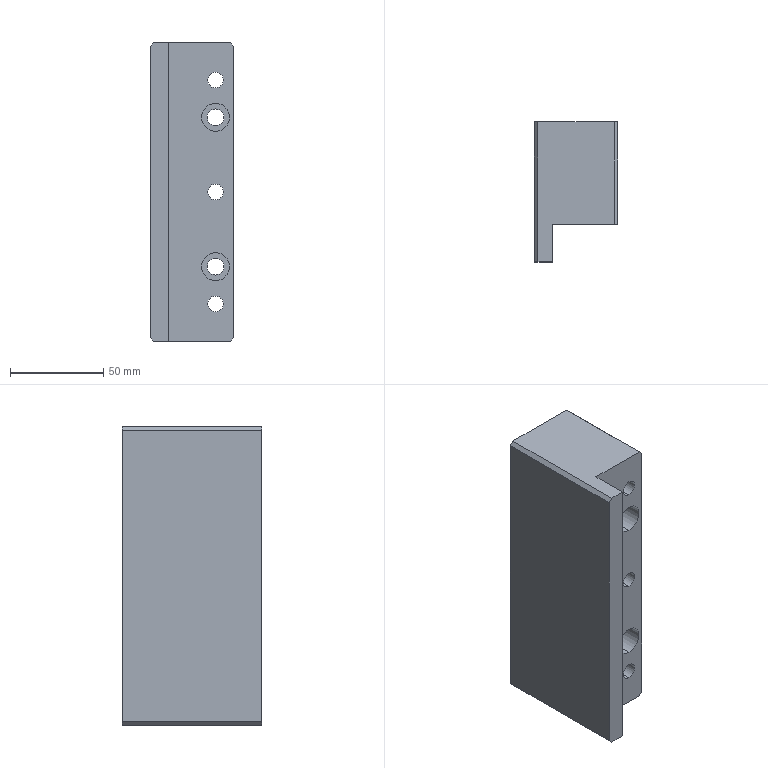Part | SolidWorks | features HoleWzd 2, Chamfer 1, Cut 1, Extrusion 1 | 1 solid | 28 faces | box 44.75 x 75 x 160 mm | volume 399871 mm3 | cylinder 14 | plane 14 | commonest cylinder face diameters 8.5 x6 9 x4 15 x4
STEP:
#1=CARTESIAN_POINT('',(12.625,60.,47.5));
#2=VERTEX_POINT('',#1);
#3=CARTESIAN_POINT('',(12.625,60.,32.5));
#4=VERTEX_POINT('',#3);
#5=CARTESIAN_POINT('',(12.625,60.,40.));
#6=DIRECTION('',(0.,-1.,0.));
#7=DIRECTION('',(0.,0.,-1.));
#8=AXIS2_PLACEMENT_3D('',#5,#6,#7);
#9=CIRCLE('',#8,7.5);
#10=EDGE_CURVE('',#2,#4,#9,.T.);
#11=ORIENTED_EDGE('',*,*,#10,.F.);
#12=CARTESIAN_POINT('',(12.625,20.,47.5));
#13=VERTEX_POINT('',#12);
#14=CARTESIAN_POINT('',(12.625,20.,47.5));
#15=DIRECTION('',(0.,-1.,0.));
#16=VECTOR('',#15,1000.);
#17=LINE('',#14,#16);
#18=EDGE_CURVE('',#2,#13,#17,.T.);
#19=ORIENTED_EDGE('',*,*,#18,.T.);
#20=CARTESIAN_POINT('',(12.625,20.,32.5));
#21=VERTEX_POINT('',#20);
#22=CARTESIAN_POINT('',(12.625,20.,40.));
#23=DIRECTION('',(0.,-1.,0.));
#24=DIRECTION('',(0.,0.,-1.));
#25=AXIS2_PLACEMENT_3D('',#22,#23,#24);
#26=CIRCLE('',#25,7.5);
#27=EDGE_CURVE('',#13,#21,#26,.T.);
#28=ORIENTED_EDGE('',*,*,#27,.T.);
#29=CARTESIAN_POINT('',(12.625,20.,32.5));
#30=DIRECTION('',(0.,-1.,0.));
#31=VECTOR('',#30,1000.);
#32=LINE('',#29,#31);
#33=EDGE_CURVE('',#4,#21,#32,.T.);
#34=ORIENTED_EDGE('',*,*,#33,.F.);
#35=EDGE_LOOP('',(#11,#19,#28,#34));
#36=FACE_OUTER_BOUND('',#35,.T.);
#37=CARTESIAN_POINT('',(12.625,20.,40.));
#38=DIRECTION('',(0.,-1.,0.));
#39=DIRECTION('',(0.,0.,-1.));
#40=AXIS2_PLACEMENT_3D('',#37,#38,#39);
#41=CYLINDRICAL_SURFACE('',#40,7.5);
#42=ADVANCED_FACE('',(#36),#41,.F.);
#43=CARTESIAN_POINT('',(12.625,75.,44.5));
#44=VERTEX_POINT('',#43);
#45=CARTESIAN_POINT('',(12.625,75.,35.5));
#46=VERTEX_POINT('',#45);
#47=CARTESIAN_POINT('',(12.625,75.,40.));
#48=DIRECTION('',(0.,-1.,0.));
#49=DIRECTION('',(0.,0.,-1.));
#50=AXIS2_PLACEMENT_3D('',#47,#48,#49);
#51=CIRCLE('',#50,4.5);
#52=EDGE_CURVE('',#44,#46,#51,.T.);
#53=ORIENTED_EDGE('',*,*,#52,.F.);
#54=CARTESIAN_POINT('',(12.625,60.,44.5));
#55=VERTEX_POINT('',#54);
#56=CARTESIAN_POINT('',(12.625,20.,44.5));
#57=DIRECTION('',(0.,-1.,0.));
#58=VECTOR('',#57,1000.);
#59=LINE('',#56,#58);
#60=EDGE_CURVE('',#44,#55,#59,.T.);
#61=ORIENTED_EDGE('',*,*,#60,.T.);
#62=CARTESIAN_POINT('',(12.625,60.,35.5));
#63=VERTEX_POINT('',#62);
#64=CARTESIAN_POINT('',(12.625,60.,40.));
#65=DIRECTION('',(0.,-1.,0.));
#66=DIRECTION('',(0.,0.,-1.));
#67=AXIS2_PLACEMENT_3D('',#64,#65,#66);
#68=CIRCLE('',#67,4.5);
#69=EDGE_CURVE('',#55,#63,#68,.T.);
#70=ORIENTED_EDGE('',*,*,#69,.T.);
#71=CARTESIAN_POINT('',(12.625,20.,35.5));
#72=DIRECTION('',(0.,-1.,0.));
#73=VECTOR('',#72,1000.);
#74=LINE('',#71,#73);
#75=EDGE_CURVE('',#46,#63,#74,.T.);
#76=ORIENTED_EDGE('',*,*,#75,.F.);
#77=EDGE_LOOP('',(#53,#61,#70,#76));
#78=FACE_OUTER_BOUND('',#77,.T.);
#79=CARTESIAN_POINT('',(12.625,20.,40.));
#80=DIRECTION('',(0.,-1.,0.));
#81=DIRECTION('',(0.,0.,-1.));
#82=AXIS2_PLACEMENT_3D('',#79,#80,#81);
#83=CYLINDRICAL_SURFACE('',#82,4.5);
#84=ADVANCED_FACE('',(#78),#83,.F.);
#85=CARTESIAN_POINT('',(12.625,60.,-32.5));
#86=VERTEX_POINT('',#85);
#87=CARTESIAN_POINT('',(12.625,60.,-47.5));
#88=VERTEX_POINT('',#87);
#89=CARTESIAN_POINT('',(12.625,60.,-40.));
#90=DIRECTION('',(0.,-1.,0.));
#91=DIRECTION('',(0.,0.,-1.));
#92=AXIS2_PLACEMENT_3D('',#89,#90,#91);
#93=CIRCLE('',#92,7.5);
#94=EDGE_CURVE('',#86,#88,#93,.T.);
#95=ORIENTED_EDGE('',*,*,#94,.F.);
#96=CARTESIAN_POINT('',(12.625,20.,-32.5));
#97=VERTEX_POINT('',#96);
#98=CARTESIAN_POINT('',(12.625,20.,-32.5));
#99=DIRECTION('',(0.,-1.,0.));
#100=VECTOR('',#99,1000.);
#101=LINE('',#98,#100);
#102=EDGE_CURVE('',#86,#97,#101,.T.);
#103=ORIENTED_EDGE('',*,*,#102,.T.);
#104=CARTESIAN_POINT('',(12.625,20.,-47.5));
#105=VERTEX_POINT('',#104);
#106=CARTESIAN_POINT('',(12.625,20.,-40.));
#107=DIRECTION('',(0.,-1.,0.));
#108=DIRECTION('',(0.,0.,-1.));
#109=AXIS2_PLACEMENT_3D('',#106,#107,#108);
#110=CIRCLE('',#109,7.5);
#111=EDGE_CURVE('',#97,#105,#110,.T.);
#112=ORIENTED_EDGE('',*,*,#111,.T.);
#113=CARTESIAN_POINT('',(12.625,20.,-47.5));
#114=DIRECTION('',(0.,-1.,0.));
#115=VECTOR('',#114,1000.);
#116=LINE('',#113,#115);
#117=EDGE_CURVE('',#88,#105,#116,.T.);
#118=ORIENTED_EDGE('',*,*,#117,.F.);
#119=EDGE_LOOP('',(#95,#103,#112,#118));
#120=FACE_OUTER_BOUND('',#119,.T.);
#121=CARTESIAN_POINT('',(12.625,20.,-40.));
#122=DIRECTION('',(0.,-1.,0.));
#123=DIRECTION('',(0.,0.,-1.));
#124=AXIS2_PLACEMENT_3D('',#121,#122,#123);
#125=CYLINDRICAL_SURFACE('',#124,7.5);
#126=ADVANCED_FACE('',(#120),#125,.F.);
#127=CARTESIAN_POINT('',(12.625,75.,-35.5));
#128=VERTEX_POINT('',#127);
#129=CARTESIAN_POINT('',(12.625,75.,-44.5));
#130=VERTEX_POINT('',#129);
#131=CARTESIAN_POINT('',(12.625,75.,-40.));
#132=DIRECTION('',(0.,-1.,0.));
#133=DIRECTION('',(0.,0.,-1.));
#134=AXIS2_PLACEMENT_3D('',#131,#132,#133);
#135=CIRCLE('',#134,4.5);
#136=EDGE_CURVE('',#128,#130,#135,.T.);
#137=ORIENTED_EDGE('',*,*,#136,.F.);
#138=CARTESIAN_POINT('',(12.625,60.,-35.5));
#139=VERTEX_POINT('',#138);
#140=CARTESIAN_POINT('',(12.625,20.,-35.5));
#141=DIRECTION('',(0.,-1.,0.));
#142=VECTOR('',#141,1000.);
#143=LINE('',#140,#142);
#144=EDGE_CURVE('',#128,#139,#143,.T.);
#145=ORIENTED_EDGE('',*,*,#144,.T.);
#146=CARTESIAN_POINT('',(12.625,60.,-44.5));
#147=VERTEX_POINT('',#146);
#148=CARTESIAN_POINT('',(12.625,60.,-40.));
#149=DIRECTION('',(0.,-1.,0.));
#150=DIRECTION('',(0.,0.,-1.));
#151=AXIS2_PLACEMENT_3D('',#148,#149,#150);
#152=CIRCLE('',#151,4.5);
#153=EDGE_CURVE('',#139,#147,#152,.T.);
#154=ORIENTED_EDGE('',*,*,#153,.T.);
#155=CARTESIAN_POINT('',(12.625,20.,-44.5));
#156=DIRECTION('',(0.,-1.,0.));
#157=VECTOR('',#156,1000.);
#158=LINE('',#155,#157);
#159=EDGE_CURVE('',#130,#147,#158,.T.);
#160=ORIENTED_EDGE('',*,*,#159,.F.);
#161=EDGE_LOOP('',(#137,#145,#154,#160));
#162=FACE_OUTER_BOUND('',#161,.T.);
#163=CARTESIAN_POINT('',(12.625,20.,-40.));
#164=DIRECTION('',(0.,-1.,0.));
#165=DIRECTION('',(0.,0.,-1.));
#166=AXIS2_PLACEMENT_3D('',#163,#164,#165);
#167=CYLINDRICAL_SURFACE('',#166,4.5);
#168=ADVANCED_FACE('',(#162),#167,.F.);
#169=CARTESIAN_POINT('',(12.625,20.,-64.25));
#170=VERTEX_POINT('',#169);
#171=CARTESIAN_POINT('',(12.625,20.,-55.75));
#172=VERTEX_POINT('',#171);
#173=CARTESIAN_POINT('',(12.625,20.,-60.));
#174=DIRECTION('',(0.,1.,0.));
#175=DIRECTION('',(0.,0.,1.));
#176=AXIS2_PLACEMENT_3D('',#173,#174,#175);
#177=CIRCLE('',#176,4.25);
#178=EDGE_CURVE('',#170,#172,#177,.T.);
#179=ORIENTED_EDGE('',*,*,#178,.F.);
#180=CARTESIAN_POINT('',(12.625,75.,-64.25));
#181=VERTEX_POINT('',#180);
#182=CARTESIAN_POINT('',(12.625,75.,-64.25));
#183=DIRECTION('',(0.,1.,0.));
#184=VECTOR('',#183,1000.);
#185=LINE('',#182,#184);
#186=EDGE_CURVE('',#170,#181,#185,.T.);
#187=ORIENTED_EDGE('',*,*,#186,.T.);
#188=CARTESIAN_POINT('',(12.625,75.,-55.75));
#189=VERTEX_POINT('',#188);
#190=CARTESIAN_POINT('',(12.625,75.,-60.));
#191=DIRECTION('',(0.,1.,0.));
#192=DIRECTION('',(0.,0.,1.));
#193=AXIS2_PLACEMENT_3D('',#190,#191,#192);
#194=CIRCLE('',#193,4.25);
#195=EDGE_CURVE('',#181,#189,#194,.T.);
#196=ORIENTED_EDGE('',*,*,#195,.T.);
#197=CARTESIAN_POINT('',(12.625,75.,-55.75));
#198=DIRECTION('',(0.,1.,0.));
#199=VECTOR('',#198,1000.);
#200=LINE('',#197,#199);
#201=EDGE_CURVE('',#172,#189,#200,.T.);
#202=ORIENTED_EDGE('',*,*,#201,.F.);
#203=EDGE_LOOP('',(#179,#187,#196,#202));
#204=FACE_OUTER_BOUND('',#203,.T.);
#205=CARTESIAN_POINT('',(12.625,75.,-60.));
#206=DIRECTION('',(0.,1.,0.));
#207=DIRECTION('',(0.,0.,1.));
#208=AXIS2_PLACEMENT_3D('',#205,#206,#207);
#209=CYLINDRICAL_SURFACE('',#208,4.25);
#210=ADVANCED_FACE('',(#204),#209,.F.);
#211=CARTESIAN_POINT('',(12.625,20.,-4.25));
#212=VERTEX_POINT('',#211);
#213=CARTESIAN_POINT('',(12.625,20.,4.25));
#214=VERTEX_POINT('',#213);
#215=CARTESIAN_POINT('',(12.625,20.,0.));
#216=DIRECTION('',(0.,1.,0.));
#217=DIRECTION('',(0.,0.,1.));
#218=AXIS2_PLACEMENT_3D('',#215,#216,#217);
#219=CIRCLE('',#218,4.25);
#220=EDGE_CURVE('',#212,#214,#219,.T.);
#221=ORIENTED_EDGE('',*,*,#220,.F.);
#222=CARTESIAN_POINT('',(12.625,75.,-4.25));
#223=VERTEX_POINT('',#222);
#224=CARTESIAN_POINT('',(12.625,75.,-4.25));
#225=DIRECTION('',(0.,1.,0.));
#226=VECTOR('',#225,1000.);
#227=LINE('',#224,#226);
#228=EDGE_CURVE('',#212,#223,#227,.T.);
#229=ORIENTED_EDGE('',*,*,#228,.T.);
#230=CARTESIAN_POINT('',(12.625,75.,4.25));
#231=VERTEX_POINT('',#230);
#232=CARTESIAN_POINT('',(12.625,75.,0.));
#233=DIRECTION('',(0.,1.,0.));
#234=DIRECTION('',(0.,0.,1.));
#235=AXIS2_PLACEMENT_3D('',#232,#233,#234);
#236=CIRCLE('',#235,4.25);
#237=EDGE_CURVE('',#223,#231,#236,.T.);
#238=ORIENTED_EDGE('',*,*,#237,.T.);
#239=CARTESIAN_POINT('',(12.625,75.,4.25));
#240=DIRECTION('',(0.,1.,0.));
#241=VECTOR('',#240,1000.);
#242=LINE('',#239,#241);
#243=EDGE_CURVE('',#214,#231,#242,.T.);
#244=ORIENTED_EDGE('',*,*,#243,.F.);
#245=EDGE_LOOP('',(#221,#229,#238,#244));
#246=FACE_OUTER_BOUND('',#245,.T.);
#247=CARTESIAN_POINT('',(12.625,75.,0.));
#248=DIRECTION('',(0.,1.,0.));
#249=DIRECTION('',(0.,0.,1.));
#250=AXIS2_PLACEMENT_3D('',#247,#248,#249);
#251=CYLINDRICAL_SURFACE('',#250,4.25);
#252=ADVANCED_FACE('',(#246),#251,.F.);
#253=CARTESIAN_POINT('',(12.625,20.,55.75));
#254=VERTEX_POINT('',#253);
#255=CARTESIAN_POINT('',(12.625,20.,64.25));
#256=VERTEX_POINT('',#255);
#257=CARTESIAN_POINT('',(12.625,20.,60.));
#258=DIRECTION('',(0.,1.,0.));
#259=DIRECTION('',(0.,0.,1.));
#260=AXIS2_PLACEMENT_3D('',#257,#258,#259);
#261=CIRCLE('',#260,4.25);
#262=EDGE_CURVE('',#254,#256,#261,.T.);
#263=ORIENTED_EDGE('',*,*,#262,.F.);
#264=CARTESIAN_POINT('',(12.625,75.,55.75));
#265=VERTEX_POINT('',#264);
#266=CARTESIAN_POINT('',(12.625,75.,55.75));
#267=DIRECTION('',(0.,1.,0.));
#268=VECTOR('',#267,1000.);
#269=LINE('',#266,#268);
#270=EDGE_CURVE('',#254,#265,#269,.T.);
#271=ORIENTED_EDGE('',*,*,#270,.T.);
#272=CARTESIAN_POINT('',(12.625,75.,64.25));
#273=VERTEX_POINT('',#272);
#274=CARTESIAN_POINT('',(12.625,75.,60.));
#275=DIRECTION('',(0.,1.,0.));
#276=DIRECTION('',(0.,0.,1.));
#277=AXIS2_PLACEMENT_3D('',#274,#275,#276);
#278=CIRCLE('',#277,4.25);
#279=EDGE_CURVE('',#265,#273,#278,.T.);
#280=ORIENTED_EDGE('',*,*,#279,.T.);
#281=CARTESIAN_POINT('',(12.625,75.,64.25));
#282=DIRECTION('',(0.,1.,0.));
#283=VECTOR('',#282,1000.);
#284=LINE('',#281,#283);
#285=EDGE_CURVE('',#256,#273,#284,.T.);
#286=ORIENTED_EDGE('',*,*,#285,.F.);
#287=EDGE_LOOP('',(#263,#271,#280,#286));
#288=FACE_OUTER_BOUND('',#287,.T.);
#289=CARTESIAN_POINT('',(12.625,75.,60.));
#290=DIRECTION('',(0.,1.,0.));
#291=DIRECTION('',(0.,0.,1.));
#292=AXIS2_PLACEMENT_3D('',#289,#290,#291);
#293=CYLINDRICAL_SURFACE('',#292,4.25);
#294=ADVANCED_FACE('',(#288),#293,.F.);
#295=CARTESIAN_POINT('',(22.375,75.,78.));
#296=VERTEX_POINT('',#295);
#297=CARTESIAN_POINT('',(22.375,75.,-78.));
#298=VERTEX_POINT('',#297);
#299=CARTESIAN_POINT('',(22.375,75.,-80.));
#300=DIRECTION('',(0.,0.,-1.));
#301=VECTOR('',#300,1000.);
#302=LINE('',#299,#301);
#303=EDGE_CURVE('',#296,#298,#302,.T.);
#304=ORIENTED_EDGE('',*,*,#303,.F.);
#305=CARTESIAN_POINT('',(22.375,20.,78.));
#306=VERTEX_POINT('',#305);
#307=CARTESIAN_POINT('',(22.375,75.,78.));
#308=DIRECTION('',(0.,-1.,0.));
#309=VECTOR('',#308,1000.);
#310=LINE('',#307,#309);
#311=EDGE_CURVE('',#296,#306,#310,.T.);
#312=ORIENTED_EDGE('',*,*,#311,.T.);
#313=CARTESIAN_POINT('',(22.375,20.,-78.));
#314=VERTEX_POINT('',#313);
#315=CARTESIAN_POINT('',(22.375,20.,80.));
#316=DIRECTION('',(0.,0.,1.));
#317=VECTOR('',#316,1000.);
#318=LINE('',#315,#317);
#319=EDGE_CURVE('',#314,#306,#318,.T.);
#320=ORIENTED_EDGE('',*,*,#319,.F.);
#321=CARTESIAN_POINT('',(22.375,75.,-78.));
#322=DIRECTION('',(0.,1.,0.));
#323=VECTOR('',#322,1000.);
#324=LINE('',#321,#323);
#325=EDGE_CURVE('',#314,#298,#324,.T.);
#326=ORIENTED_EDGE('',*,*,#325,.T.);
#327=EDGE_LOOP('',(#304,#312,#320,#326));
#328=FACE_OUTER_BOUND('',#327,.T.);
#329=CARTESIAN_POINT('',(22.375,75.,-80.));
#330=DIRECTION('',(-1.,0.,0.));
#331=DIRECTION('',(0.,0.,1.));
#332=AXIS2_PLACEMENT_3D('',#329,#330,#331);
#333=PLANE('',#332);
#334=ADVANCED_FACE('',(#328),#333,.F.);
#335=CARTESIAN_POINT('',(20.375,75.,-80.));
#336=VERTEX_POINT('',#335);
#337=CARTESIAN_POINT('',(-20.375,75.,-80.));
#338=VERTEX_POINT('',#337);
#339=CARTESIAN_POINT('',(-22.375,75.,-80.));
#340=DIRECTION('',(-1.,0.,0.));
#341=VECTOR('',#340,1000.);
#342=LINE('',#339,#341);
#343=EDGE_CURVE('',#336,#338,#342,.T.);
#344=ORIENTED_EDGE('',*,*,#343,.F.);
#345=CARTESIAN_POINT('',(20.375,20.,-80.));
#346=VERTEX_POINT('',#345);
#347=CARTESIAN_POINT('',(20.375,75.,-80.));
#348=DIRECTION('',(0.,-1.,0.));
#349=VECTOR('',#348,1000.);
#350=LINE('',#347,#349);
#351=EDGE_CURVE('',#336,#346,#350,.T.);
#352=ORIENTED_EDGE('',*,*,#351,.T.);
#353=CARTESIAN_POINT('',(-12.375,20.,-80.));
#354=VERTEX_POINT('',#353);
#355=CARTESIAN_POINT('',(22.375,20.,-80.));
#356=DIRECTION('',(1.,0.,0.));
#357=VECTOR('',#356,1000.);
#358=LINE('',#355,#357);
#359=EDGE_CURVE('',#354,#346,#358,.T.);
#360=ORIENTED_EDGE('',*,*,#359,.F.);
#361=CARTESIAN_POINT('',(-12.375,0.,-80.));
#362=VERTEX_POINT('',#361);
#363=CARTESIAN_POINT('',(-12.375,20.,-80.));
#364=DIRECTION('',(0.,-1.,0.));
#365=VECTOR('',#364,1000.);
#366=LINE('',#363,#365);
#367=EDGE_CURVE('',#354,#362,#366,.T.);
#368=ORIENTED_EDGE('',*,*,#367,.T.);
#369=CARTESIAN_POINT('',(-20.375,0.,-80.));
#370=VERTEX_POINT('',#369);
#371=CARTESIAN_POINT('',(-22.375,0.,-80.));
#372=DIRECTION('',(-1.,0.,0.));
#373=VECTOR('',#372,1000.);
#374=LINE('',#371,#373);
#375=EDGE_CURVE('',#362,#370,#374,.T.);
#376=ORIENTED_EDGE('',*,*,#375,.T.);
#377=CARTESIAN_POINT('',(-20.375,75.,-80.));
#378=DIRECTION('',(0.,1.,0.));
#379=VECTOR('',#378,1000.);
#380=LINE('',#377,#379);
#381=EDGE_CURVE('',#370,#338,#380,.T.);
#382=ORIENTED_EDGE('',*,*,#381,.T.);
#383=EDGE_LOOP('',(#344,#352,#360,#368,#376,#382));
#384=FACE_OUTER_BOUND('',#383,.T.);
#385=CARTESIAN_POINT('',(-22.375,75.,-80.));
#386=DIRECTION('',(0.,0.,1.));
#387=DIRECTION('',(1.,0.,0.));
#388=AXIS2_PLACEMENT_3D('',#385,#386,#387);
#389=PLANE('',#388);
#390=ADVANCED_FACE('',(#384),#389,.F.);
#391=CARTESIAN_POINT('',(-22.375,0.,-78.));
#392=VERTEX_POINT('',#391);
#393=CARTESIAN_POINT('',(-22.375,0.,78.));
#394=VERTEX_POINT('',#393);
#395=CARTESIAN_POINT('',(-22.375,0.,-80.));
#396=DIRECTION('',(0.,0.,1.));
#397=VECTOR('',#396,1000.);
#398=LINE('',#395,#397);
#399=EDGE_CURVE('',#392,#394,#398,.T.);
#400=ORIENTED_EDGE('',*,*,#399,.T.);
#401=CARTESIAN_POINT('',(-22.375,75.,78.));
#402=VERTEX_POINT('',#401);
#403=CARTESIAN_POINT('',(-22.375,75.,78.));
#404=DIRECTION('',(0.,1.,0.));
#405=VECTOR('',#404,1000.);
#406=LINE('',#403,#405);
#407=EDGE_CURVE('',#394,#402,#406,.T.);
#408=ORIENTED_EDGE('',*,*,#407,.T.);
#409=CARTESIAN_POINT('',(-22.375,75.,-78.));
#410=VERTEX_POINT('',#409);
#411=CARTESIAN_POINT('',(-22.375,75.,-80.));
#412=DIRECTION('',(0.,0.,1.));
#413=VECTOR('',#412,1000.);
#414=LINE('',#411,#413);
#415=EDGE_CURVE('',#410,#402,#414,.T.);
#416=ORIENTED_EDGE('',*,*,#415,.F.);
#417=CARTESIAN_POINT('',(-22.375,75.,-78.));
#418=DIRECTION('',(0.,-1.,0.));
#419=VECTOR('',#418,1000.);
#420=LINE('',#417,#419);
#421=EDGE_CURVE('',#410,#392,#420,.T.);
#422=ORIENTED_EDGE('',*,*,#421,.T.);
#423=EDGE_LOOP('',(#400,#408,#416,#422));
#424=FACE_OUTER_BOUND('',#423,.T.);
#425=CARTESIAN_POINT('',(-22.375,75.,-80.));
#426=DIRECTION('',(1.,0.,0.));
#427=DIRECTION('',(0.,0.,-1.));
#428=AXIS2_PLACEMENT_3D('',#425,#426,#427);
#429=PLANE('',#428);
#430=ADVANCED_FACE('',(#424),#429,.F.);
#431=CARTESIAN_POINT('',(-20.375,75.,80.));
#432=VERTEX_POINT('',#431);
#433=CARTESIAN_POINT('',(20.375,75.,80.));
#434=VERTEX_POINT('',#433);
#435=CARTESIAN_POINT('',(-22.375,75.,80.));
#436=DIRECTION('',(1.,0.,0.));
#437=VECTOR('',#436,1000.);
#438=LINE('',#435,#437);
#439=EDGE_CURVE('',#432,#434,#438,.T.);
#440=ORIENTED_EDGE('',*,*,#439,.F.);
#441=CARTESIAN_POINT('',(-20.375,0.,80.));
#442=VERTEX_POINT('',#441);
#443=CARTESIAN_POINT('',(-20.375,75.,80.));
#444=DIRECTION('',(0.,-1.,0.));
#445=VECTOR('',#444,1000.);
#446=LINE('',#443,#445);
#447=EDGE_CURVE('',#432,#442,#446,.T.);
#448=ORIENTED_EDGE('',*,*,#447,.T.);
#449=CARTESIAN_POINT('',(-12.375,0.,80.));
#450=VERTEX_POINT('',#449);
#451=CARTESIAN_POINT('',(-22.375,0.,80.));
#452=DIRECTION('',(1.,0.,0.));
#453=VECTOR('',#452,1000.);
#454=LINE('',#451,#453);
#455=EDGE_CURVE('',#442,#450,#454,.T.);
#456=ORIENTED_EDGE('',*,*,#455,.T.);
#457=CARTESIAN_POINT('',(-12.375,20.,80.));
#458=VERTEX_POINT('',#457);
#459=CARTESIAN_POINT('',(-12.375,20.,80.));
#460=DIRECTION('',(0.,-1.,0.));
#461=VECTOR('',#460,1000.);
#462=LINE('',#459,#461);
#463=EDGE_CURVE('',#458,#450,#462,.T.);
#464=ORIENTED_EDGE('',*,*,#463,.F.);
#465=CARTESIAN_POINT('',(20.375,20.,80.));
#466=VERTEX_POINT('',#465);
#467=CARTESIAN_POINT('',(22.375,20.,80.));
#468=DIRECTION('',(-1.,0.,0.));
#469=VECTOR('',#468,1000.);
#470=LINE('',#467,#469);
#471=EDGE_CURVE('',#466,#458,#470,.T.);
#472=ORIENTED_EDGE('',*,*,#471,.F.);
#473=CARTESIAN_POINT('',(20.375,75.,80.));
#474=DIRECTION('',(0.,1.,0.));
#475=VECTOR('',#474,1000.);
#476=LINE('',#473,#475);
#477=EDGE_CURVE('',#466,#434,#476,.T.);
#478=ORIENTED_EDGE('',*,*,#477,.T.);
#479=EDGE_LOOP('',(#440,#448,#456,#464,#472,#478));
#480=FACE_OUTER_BOUND('',#479,.T.);
#481=CARTESIAN_POINT('',(-22.375,75.,80.));
#482=DIRECTION('',(0.,0.,-1.));
#483=DIRECTION('',(-1.,0.,0.));
#484=AXIS2_PLACEMENT_3D('',#481,#482,#483);
#485=PLANE('',#484);
#486=ADVANCED_FACE('',(#480),#485,.F.);
#487=CARTESIAN_POINT('',(12.625,75.,40.));
#488=DIRECTION('',(0.,-1.,0.));
#489=DIRECTION('',(0.,0.,-1.));
#490=AXIS2_PLACEMENT_3D('',#487,#488,#489);
#491=CIRCLE('',#490,4.5);
#492=EDGE_CURVE('',#46,#44,#491,.T.);
#493=ORIENTED_EDGE('',*,*,#492,.T.);
#494=ORIENTED_EDGE('',*,*,#52,.T.);
#495=EDGE_LOOP('',(#493,#494));
#496=FACE_BOUND('',#495,.T.);
#497=CARTESIAN_POINT('',(12.625,75.,-40.));
#498=DIRECTION('',(0.,-1.,0.));
#499=DIRECTION('',(0.,0.,-1.));
#500=AXIS2_PLACEMENT_3D('',#497,#498,#499);
#501=CIRCLE('',#500,4.5);
#502=EDGE_CURVE('',#130,#128,#501,.T.);
#503=ORIENTED_EDGE('',*,*,#502,.T.);
#504=ORIENTED_EDGE('',*,*,#136,.T.);
#505=EDGE_LOOP('',(#503,#504));
#506=FACE_BOUND('',#505,.T.);
#507=CARTESIAN_POINT('',(12.625,75.,-60.));
#508=DIRECTION('',(0.,1.,0.));
#509=DIRECTION('',(0.,0.,1.));
#510=AXIS2_PLACEMENT_3D('',#507,#508,#509);
#511=CIRCLE('',#510,4.25);
#512=EDGE_CURVE('',#189,#181,#511,.T.);
#513=ORIENTED_EDGE('',*,*,#512,.F.);
#514=ORIENTED_EDGE('',*,*,#195,.F.);
#515=EDGE_LOOP('',(#513,#514));
#516=FACE_BOUND('',#515,.T.);
#517=CARTESIAN_POINT('',(12.625,75.,0.));
#518=DIRECTION('',(0.,1.,0.));
#519=DIRECTION('',(0.,0.,1.));
#520=AXIS2_PLACEMENT_3D('',#517,#518,#519);
#521=CIRCLE('',#520,4.25);
#522=EDGE_CURVE('',#231,#223,#521,.T.);
#523=ORIENTED_EDGE('',*,*,#522,.F.);
#524=ORIENTED_EDGE('',*,*,#237,.F.);
#525=EDGE_LOOP('',(#523,#524));
#526=FACE_BOUND('',#525,.T.);
#527=CARTESIAN_POINT('',(12.625,75.,60.));
#528=DIRECTION('',(0.,1.,0.));
#529=DIRECTION('',(0.,0.,1.));
#530=AXIS2_PLACEMENT_3D('',#527,#528,#529);
#531=CIRCLE('',#530,4.25);
#532=EDGE_CURVE('',#273,#265,#531,.T.);
#533=ORIENTED_EDGE('',*,*,#532,.F.);
#534=ORIENTED_EDGE('',*,*,#279,.F.);
#535=EDGE_LOOP('',(#533,#534));
#536=FACE_BOUND('',#535,.T.);
#537=ORIENTED_EDGE('',*,*,#415,.T.);
#538=CARTESIAN_POINT('',(-50.187,75.,50.187));
#539=DIRECTION('',(0.7071,0.,0.7071));
#540=VECTOR('',#539,1000.);
#541=LINE('',#538,#540);
#542=EDGE_CURVE('',#402,#432,#541,.T.);
#543=ORIENTED_EDGE('',*,*,#542,.T.);
#544=ORIENTED_EDGE('',*,*,#439,.T.);
#545=CARTESIAN_POINT('',(50.188,75.,50.187));
#546=DIRECTION('',(0.7071,0.,-0.7071));
#547=VECTOR('',#546,1000.);
#548=LINE('',#545,#547);
#549=EDGE_CURVE('',#434,#296,#548,.T.);
#550=ORIENTED_EDGE('',*,*,#549,.T.);
#551=ORIENTED_EDGE('',*,*,#303,.T.);
#552=CARTESIAN_POINT('',(50.187,75.,-50.187));
#553=DIRECTION('',(-0.7071,0.,-0.7071));
#554=VECTOR('',#553,1000.);
#555=LINE('',#552,#554);
#556=EDGE_CURVE('',#298,#336,#555,.T.);
#557=ORIENTED_EDGE('',*,*,#556,.T.);
#558=ORIENTED_EDGE('',*,*,#343,.T.);
#559=CARTESIAN_POINT('',(-50.188,75.,-50.188));
#560=DIRECTION('',(-0.7071,0.,0.7071));
#561=VECTOR('',#560,1000.);
#562=LINE('',#559,#561);
#563=EDGE_CURVE('',#338,#410,#562,.T.);
#564=ORIENTED_EDGE('',*,*,#563,.T.);
#565=EDGE_LOOP('',(#537,#543,#544,#550,#551,#557,#558,#564));
#566=FACE_OUTER_BOUND('',#565,.T.);
#567=CARTESIAN_POINT('',(0.,75.,0.));
#568=DIRECTION('',(0.,1.,0.));
#569=DIRECTION('',(0.,0.,1.));
#570=AXIS2_PLACEMENT_3D('',#567,#568,#569);
#571=PLANE('',#570);
#572=ADVANCED_FACE('',(#496,#506,#516,#526,#536,#566),#571,.T.);
#573=ORIENTED_EDGE('',*,*,#455,.F.);
#574=CARTESIAN_POINT('',(-20.375,0.,80.));
#575=DIRECTION('',(-0.7071,0.,-0.7071));
#576=VECTOR('',#575,1000.);
#577=LINE('',#574,#576);
#578=EDGE_CURVE('',#442,#394,#577,.T.);
#579=ORIENTED_EDGE('',*,*,#578,.T.);
#580=ORIENTED_EDGE('',*,*,#399,.F.);
#581=CARTESIAN_POINT('',(-22.375,0.,-78.));
#582=DIRECTION('',(0.7071,0.,-0.7071));
#583=VECTOR('',#582,1000.);
#584=LINE('',#581,#583);
#585=EDGE_CURVE('',#392,#370,#584,.T.);
#586=ORIENTED_EDGE('',*,*,#585,.T.);
#587=ORIENTED_EDGE('',*,*,#375,.F.);
#588=CARTESIAN_POINT('',(-12.375,0.,80.));
#589=DIRECTION('',(0.,0.,-1.));
#590=VECTOR('',#589,1000.);
#591=LINE('',#588,#590);
#592=EDGE_CURVE('',#450,#362,#591,.T.);
#593=ORIENTED_EDGE('',*,*,#592,.F.);
#594=EDGE_LOOP('',(#573,#579,#580,#586,#587,#593));
#595=FACE_OUTER_BOUND('',#594,.T.);
#596=CARTESIAN_POINT('',(0.,0.,0.));
#597=DIRECTION('',(0.,1.,0.));
#598=DIRECTION('',(0.,0.,1.));
#599=AXIS2_PLACEMENT_3D('',#596,#597,#598);
#600=PLANE('',#599);
#601=ADVANCED_FACE('',(#595),#600,.F.);
#602=ORIENTED_EDGE('',*,*,#592,.T.);
#603=ORIENTED_EDGE('',*,*,#367,.F.);
#604=CARTESIAN_POINT('',(-12.375,20.,80.));
#605=DIRECTION('',(0.,0.,-1.));
#606=VECTOR('',#605,1000.);
#607=LINE('',#604,#606);
#608=EDGE_CURVE('',#458,#354,#607,.T.);
#609=ORIENTED_EDGE('',*,*,#608,.F.);
#610=ORIENTED_EDGE('',*,*,#463,.T.);
#611=EDGE_LOOP('',(#602,#603,#609,#610));
#612=FACE_OUTER_BOUND('',#611,.T.);
#613=CARTESIAN_POINT('',(-12.375,20.,80.));
#614=DIRECTION('',(-1.,0.,0.));
#615=DIRECTION('',(0.,0.,1.));
#616=AXIS2_PLACEMENT_3D('',#613,#614,#615);
#617=PLANE('',#616);
#618=ADVANCED_FACE('',(#612),#617,.F.);
#619=CARTESIAN_POINT('',(12.625,20.,40.));
#620=DIRECTION('',(0.,-1.,0.));
#621=DIRECTION('',(0.,0.,-1.));
#622=AXIS2_PLACEMENT_3D('',#619,#620,#621);
#623=CIRCLE('',#622,7.5);
#624=EDGE_CURVE('',#21,#13,#623,.T.);
#625=ORIENTED_EDGE('',*,*,#624,.F.);
#626=ORIENTED_EDGE('',*,*,#27,.F.);
#627=EDGE_LOOP('',(#625,#626));
#628=FACE_BOUND('',#627,.T.);
#629=CARTESIAN_POINT('',(12.625,20.,-40.));
#630=DIRECTION('',(0.,-1.,0.));
#631=DIRECTION('',(0.,0.,-1.));
#632=AXIS2_PLACEMENT_3D('',#629,#630,#631);
#633=CIRCLE('',#632,7.5);
#634=EDGE_CURVE('',#105,#97,#633,.T.);
#635=ORIENTED_EDGE('',*,*,#634,.F.);
#636=ORIENTED_EDGE('',*,*,#111,.F.);
#637=EDGE_LOOP('',(#635,#636));
#638=FACE_BOUND('',#637,.T.);
#639=CARTESIAN_POINT('',(12.625,20.,-60.));
#640=DIRECTION('',(0.,1.,0.));
#641=DIRECTION('',(0.,0.,1.));
#642=AXIS2_PLACEMENT_3D('',#639,#640,#641);
#643=CIRCLE('',#642,4.25);
#644=EDGE_CURVE('',#172,#170,#643,.T.);
#645=ORIENTED_EDGE('',*,*,#644,.T.);
#646=ORIENTED_EDGE('',*,*,#178,.T.);
#647=EDGE_LOOP('',(#645,#646));
#648=FACE_BOUND('',#647,.T.);
#649=CARTESIAN_POINT('',(12.625,20.,0.));
#650=DIRECTION('',(0.,1.,0.));
#651=DIRECTION('',(0.,0.,1.));
#652=AXIS2_PLACEMENT_3D('',#649,#650,#651);
#653=CIRCLE('',#652,4.25);
#654=EDGE_CURVE('',#214,#212,#653,.T.);
#655=ORIENTED_EDGE('',*,*,#654,.T.);
#656=ORIENTED_EDGE('',*,*,#220,.T.);
#657=EDGE_LOOP('',(#655,#656));
#658=FACE_BOUND('',#657,.T.);
#659=CARTESIAN_POINT('',(12.625,20.,60.));
#660=DIRECTION('',(0.,1.,0.));
#661=DIRECTION('',(0.,0.,1.));
#662=AXIS2_PLACEMENT_3D('',#659,#660,#661);
#663=CIRCLE('',#662,4.25);
#664=EDGE_CURVE('',#256,#254,#663,.T.);
#665=ORIENTED_EDGE('',*,*,#664,.T.);
#666=ORIENTED_EDGE('',*,*,#262,.T.);
#667=EDGE_LOOP('',(#665,#666));
#668=FACE_BOUND('',#667,.T.);
#669=ORIENTED_EDGE('',*,*,#319,.T.);
#670=CARTESIAN_POINT('',(22.375,20.,78.));
#671=DIRECTION('',(-0.7071,0.,0.7071));
#672=VECTOR('',#671,1000.);
#673=LINE('',#670,#672);
#674=EDGE_CURVE('',#306,#466,#673,.T.);
#675=ORIENTED_EDGE('',*,*,#674,.T.);
#676=ORIENTED_EDGE('',*,*,#471,.T.);
#677=ORIENTED_EDGE('',*,*,#608,.T.);
#678=ORIENTED_EDGE('',*,*,#359,.T.);
#679=CARTESIAN_POINT('',(20.375,20.,-80.));
#680=DIRECTION('',(0.7071,0.,0.7071));
#681=VECTOR('',#680,1000.);
#682=LINE('',#679,#681);
#683=EDGE_CURVE('',#346,#314,#682,.T.);
#684=ORIENTED_EDGE('',*,*,#683,.T.);
#685=EDGE_LOOP('',(#669,#675,#676,#677,#678,#684));
#686=FACE_OUTER_BOUND('',#685,.T.);
#687=CARTESIAN_POINT('',(0.,20.,0.));
#688=DIRECTION('',(0.,1.,0.));
#689=DIRECTION('',(0.,0.,1.));
#690=AXIS2_PLACEMENT_3D('',#687,#688,#689);
#691=PLANE('',#690);
#692=ADVANCED_FACE('',(#628,#638,#648,#658,#668,#686),#691,.F.);
#693=ORIENTED_EDGE('',*,*,#270,.F.);
#694=ORIENTED_EDGE('',*,*,#664,.F.);
#695=ORIENTED_EDGE('',*,*,#285,.T.);
#696=ORIENTED_EDGE('',*,*,#532,.T.);
#697=EDGE_LOOP('',(#693,#694,#695,#696));
#698=FACE_OUTER_BOUND('',#697,.T.);
#699=CARTESIAN_POINT('',(12.625,75.,60.));
#700=DIRECTION('',(0.,1.,0.));
#701=DIRECTION('',(0.,0.,1.));
#702=AXIS2_PLACEMENT_3D('',#699,#700,#701);
#703=CYLINDRICAL_SURFACE('',#702,4.25);
#704=ADVANCED_FACE('',(#698),#703,.F.);
#705=ORIENTED_EDGE('',*,*,#228,.F.);
#706=ORIENTED_EDGE('',*,*,#654,.F.);
#707=ORIENTED_EDGE('',*,*,#243,.T.);
#708=ORIENTED_EDGE('',*,*,#522,.T.);
#709=EDGE_LOOP('',(#705,#706,#707,#708));
#710=FACE_OUTER_BOUND('',#709,.T.);
#711=CARTESIAN_POINT('',(12.625,75.,0.));
#712=DIRECTION('',(0.,1.,0.));
#713=DIRECTION('',(0.,0.,1.));
#714=AXIS2_PLACEMENT_3D('',#711,#712,#713);
#715=CYLINDRICAL_SURFACE('',#714,4.25);
#716=ADVANCED_FACE('',(#710),#715,.F.);
#717=ORIENTED_EDGE('',*,*,#186,.F.);
#718=ORIENTED_EDGE('',*,*,#644,.F.);
#719=ORIENTED_EDGE('',*,*,#201,.T.);
#720=ORIENTED_EDGE('',*,*,#512,.T.);
#721=EDGE_LOOP('',(#717,#718,#719,#720));
#722=FACE_OUTER_BOUND('',#721,.T.);
#723=CARTESIAN_POINT('',(12.625,75.,-60.));
#724=DIRECTION('',(0.,1.,0.));
#725=DIRECTION('',(0.,0.,1.));
#726=AXIS2_PLACEMENT_3D('',#723,#724,#725);
#727=CYLINDRICAL_SURFACE('',#726,4.25);
#728=ADVANCED_FACE('',(#722),#727,.F.);
#729=ORIENTED_EDGE('',*,*,#542,.F.);
#730=ORIENTED_EDGE('',*,*,#407,.F.);
#731=ORIENTED_EDGE('',*,*,#578,.F.);
#732=ORIENTED_EDGE('',*,*,#447,.F.);
#733=EDGE_LOOP('',(#729,#730,#731,#732));
#734=FACE_OUTER_BOUND('',#733,.T.);
#735=CARTESIAN_POINT('',(-20.375,75.,80.));
#736=DIRECTION('',(0.7071,0.,-0.7071));
#737=DIRECTION('',(0.,-1.,0.));
#738=AXIS2_PLACEMENT_3D('',#735,#736,#737);
#739=PLANE('',#738);
#740=ADVANCED_FACE('',(#734),#739,.F.);
#741=ORIENTED_EDGE('',*,*,#549,.F.);
#742=ORIENTED_EDGE('',*,*,#477,.F.);
#743=ORIENTED_EDGE('',*,*,#674,.F.);
#744=ORIENTED_EDGE('',*,*,#311,.F.);
#745=EDGE_LOOP('',(#741,#742,#743,#744));
#746=FACE_OUTER_BOUND('',#745,.T.);
#747=CARTESIAN_POINT('',(22.375,75.,78.));
#748=DIRECTION('',(-0.7071,0.,-0.7071));
#749=DIRECTION('',(0.,-1.,0.));
#750=AXIS2_PLACEMENT_3D('',#747,#748,#749);
#751=PLANE('',#750);
#752=ADVANCED_FACE('',(#746),#751,.F.);
#753=ORIENTED_EDGE('',*,*,#556,.F.);
#754=ORIENTED_EDGE('',*,*,#325,.F.);
#755=ORIENTED_EDGE('',*,*,#683,.F.);
#756=ORIENTED_EDGE('',*,*,#351,.F.);
#757=EDGE_LOOP('',(#753,#754,#755,#756));
#758=FACE_OUTER_BOUND('',#757,.T.);
#759=CARTESIAN_POINT('',(20.375,75.,-80.));
#760=DIRECTION('',(-0.7071,0.,0.7071));
#761=DIRECTION('',(0.,-1.,0.));
#762=AXIS2_PLACEMENT_3D('',#759,#760,#761);
#763=PLANE('',#762);
#764=ADVANCED_FACE('',(#758),#763,.F.);
#765=ORIENTED_EDGE('',*,*,#563,.F.);
#766=ORIENTED_EDGE('',*,*,#381,.F.);
#767=ORIENTED_EDGE('',*,*,#585,.F.);
#768=ORIENTED_EDGE('',*,*,#421,.F.);
#769=EDGE_LOOP('',(#765,#766,#767,#768));
#770=FACE_OUTER_BOUND('',#769,.T.);
#771=CARTESIAN_POINT('',(-22.375,75.,-78.));
#772=DIRECTION('',(0.7071,0.,0.7071));
#773=DIRECTION('',(0.,-1.,0.));
#774=AXIS2_PLACEMENT_3D('',#771,#772,#773);
#775=PLANE('',#774);
#776=ADVANCED_FACE('',(#770),#775,.F.);
#777=ORIENTED_EDGE('',*,*,#144,.F.);
#778=ORIENTED_EDGE('',*,*,#502,.F.);
#779=ORIENTED_EDGE('',*,*,#159,.T.);
#780=CARTESIAN_POINT('',(12.625,60.,-40.));
#781=DIRECTION('',(0.,-1.,0.));
#782=DIRECTION('',(0.,0.,-1.));
#783=AXIS2_PLACEMENT_3D('',#780,#781,#782);
#784=CIRCLE('',#783,4.5);
#785=EDGE_CURVE('',#147,#139,#784,.T.);
#786=ORIENTED_EDGE('',*,*,#785,.T.);
#787=EDGE_LOOP('',(#777,#778,#779,#786));
#788=FACE_OUTER_BOUND('',#787,.T.);
#789=CARTESIAN_POINT('',(12.625,20.,-40.));
#790=DIRECTION('',(0.,-1.,0.));
#791=DIRECTION('',(0.,0.,-1.));
#792=AXIS2_PLACEMENT_3D('',#789,#790,#791);
#793=CYLINDRICAL_SURFACE('',#792,4.5);
#794=ADVANCED_FACE('',(#788),#793,.F.);
#795=ORIENTED_EDGE('',*,*,#785,.F.);
#796=ORIENTED_EDGE('',*,*,#153,.F.);
#797=EDGE_LOOP('',(#795,#796));
#798=FACE_BOUND('',#797,.T.);
#799=CARTESIAN_POINT('',(12.625,60.,-40.));
#800=DIRECTION('',(0.,-1.,0.));
#801=DIRECTION('',(0.,0.,-1.));
#802=AXIS2_PLACEMENT_3D('',#799,#800,#801);
#803=CIRCLE('',#802,7.5);
#804=EDGE_CURVE('',#88,#86,#803,.T.);
#805=ORIENTED_EDGE('',*,*,#804,.T.);
#806=ORIENTED_EDGE('',*,*,#94,.T.);
#807=EDGE_LOOP('',(#805,#806));
#808=FACE_OUTER_BOUND('',#807,.T.);
#809=CARTESIAN_POINT('',(17.125,60.,-40.));
#810=DIRECTION('',(0.,1.,0.));
#811=DIRECTION('',(0.,0.,1.));
#812=AXIS2_PLACEMENT_3D('',#809,#810,#811);
#813=PLANE('',#812);
#814=ADVANCED_FACE('',(#798,#808),#813,.F.);
#815=ORIENTED_EDGE('',*,*,#102,.F.);
#816=ORIENTED_EDGE('',*,*,#804,.F.);
#817=ORIENTED_EDGE('',*,*,#117,.T.);
#818=ORIENTED_EDGE('',*,*,#634,.T.);
#819=EDGE_LOOP('',(#815,#816,#817,#818));
#820=FACE_OUTER_BOUND('',#819,.T.);
#821=CARTESIAN_POINT('',(12.625,20.,-40.));
#822=DIRECTION('',(0.,-1.,0.));
#823=DIRECTION('',(0.,0.,-1.));
#824=AXIS2_PLACEMENT_3D('',#821,#822,#823);
#825=CYLINDRICAL_SURFACE('',#824,7.5);
#826=ADVANCED_FACE('',(#820),#825,.F.);
#827=ORIENTED_EDGE('',*,*,#60,.F.);
#828=ORIENTED_EDGE('',*,*,#492,.F.);
#829=ORIENTED_EDGE('',*,*,#75,.T.);
#830=CARTESIAN_POINT('',(12.625,60.,40.));
#831=DIRECTION('',(0.,-1.,0.));
#832=DIRECTION('',(0.,0.,-1.));
#833=AXIS2_PLACEMENT_3D('',#830,#831,#832);
#834=CIRCLE('',#833,4.5);
#835=EDGE_CURVE('',#63,#55,#834,.T.);
#836=ORIENTED_EDGE('',*,*,#835,.T.);
#837=EDGE_LOOP('',(#827,#828,#829,#836));
#838=FACE_OUTER_BOUND('',#837,.T.);
#839=CARTESIAN_POINT('',(12.625,20.,40.));
#840=DIRECTION('',(0.,-1.,0.));
#841=DIRECTION('',(0.,0.,-1.));
#842=AXIS2_PLACEMENT_3D('',#839,#840,#841);
#843=CYLINDRICAL_SURFACE('',#842,4.5);
#844=ADVANCED_FACE('',(#838),#843,.F.);
#845=ORIENTED_EDGE('',*,*,#835,.F.);
#846=ORIENTED_EDGE('',*,*,#69,.F.);
#847=EDGE_LOOP('',(#845,#846));
#848=FACE_BOUND('',#847,.T.);
#849=CARTESIAN_POINT('',(12.625,60.,40.));
#850=DIRECTION('',(0.,-1.,0.));
#851=DIRECTION('',(0.,0.,-1.));
#852=AXIS2_PLACEMENT_3D('',#849,#850,#851);
#853=CIRCLE('',#852,7.5);
#854=EDGE_CURVE('',#4,#2,#853,.T.);
#855=ORIENTED_EDGE('',*,*,#854,.T.);
#856=ORIENTED_EDGE('',*,*,#10,.T.);
#857=EDGE_LOOP('',(#855,#856));
#858=FACE_OUTER_BOUND('',#857,.T.);
#859=CARTESIAN_POINT('',(17.125,60.,40.));
#860=DIRECTION('',(0.,1.,0.));
#861=DIRECTION('',(0.,0.,1.));
#862=AXIS2_PLACEMENT_3D('',#859,#860,#861);
#863=PLANE('',#862);
#864=ADVANCED_FACE('',(#848,#858),#863,.F.);
#865=ORIENTED_EDGE('',*,*,#18,.F.);
#866=ORIENTED_EDGE('',*,*,#854,.F.);
#867=ORIENTED_EDGE('',*,*,#33,.T.);
#868=ORIENTED_EDGE('',*,*,#624,.T.);
#869=EDGE_LOOP('',(#865,#866,#867,#868));
#870=FACE_OUTER_BOUND('',#869,.T.);
#871=CARTESIAN_POINT('',(12.625,20.,40.));
#872=DIRECTION('',(0.,-1.,0.));
#873=DIRECTION('',(0.,0.,-1.));
#874=AXIS2_PLACEMENT_3D('',#871,#872,#873);
#875=CYLINDRICAL_SURFACE('',#874,7.5);
#876=ADVANCED_FACE('',(#870),#875,.F.);
#877=CLOSED_SHELL('',(#42,#84,#126,#168,#210,#252,#294,#334,#390,#430,#486,#572,#601,#618,#692,#704,#716,#728,#740,#752,#764,#776,#794,#814,#826,#844,#864,#876));
#878=MANIFOLD_SOLID_BREP('',#877);
#879=CARTESIAN_POINT('',(0.,0.,0.));
#880=DIRECTION('',(0.,0.,1.));
#881=DIRECTION('',(1.,0.,0.));
#882=AXIS2_PLACEMENT_3D('',#879,#880,#881);
#883=(LENGTH_UNIT()NAMED_UNIT(*)SI_UNIT(.MILLI.,.METRE.));
#884=UNCERTAINTY_MEASURE_WITH_UNIT(LENGTH_MEASURE(0.00001),#883,'','');
#885=(NAMED_UNIT(*)PLANE_ANGLE_UNIT()SI_UNIT($,.RADIAN.));
#886=(NAMED_UNIT(*)SI_UNIT($,.STERADIAN.)SOLID_ANGLE_UNIT());
#887=(GEOMETRIC_REPRESENTATION_CONTEXT(3)GLOBAL_UNCERTAINTY_ASSIGNED_CONTEXT((#884))GLOBAL_UNIT_ASSIGNED_CONTEXT((#883,#885,#886))REPRESENTATION_CONTEXT('',''));
#888=ADVANCED_BREP_SHAPE_REPRESENTATION('',(#878,#882),#887);